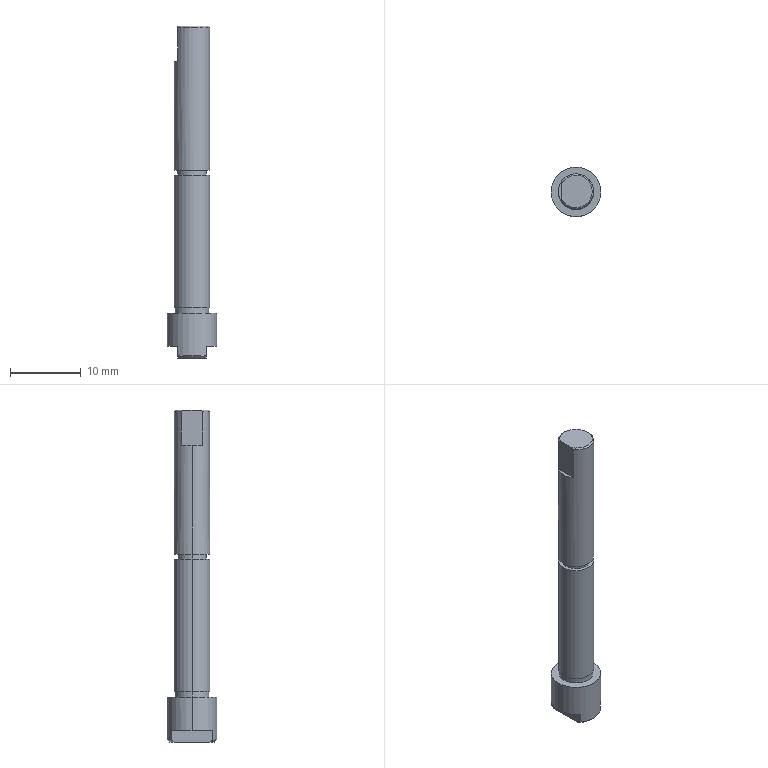Part | NX | 1 solid | 31 faces | box 7 x 7 x 46.9 mm | volume 962.4 mm3 | plane 12 | cylinder 12 | cone 7 | commonest cylinder face diameters 5 x4 2.5 x2 4 x2 4.8 x2 7 x2
STEP:
#1=CARTESIAN_POINT('',(-2.,1.136,41.07));
#2=VERTEX_POINT('',#1);
#3=CARTESIAN_POINT('',(-2.,-1.136,41.07));
#4=VERTEX_POINT('',#3);
#5=CARTESIAN_POINT('',(0.,0.,41.07));
#6=DIRECTION('',(0.,0.,-1.));
#7=DIRECTION('',(-1.,0.,0.));
#8=AXIS2_PLACEMENT_3D('',#5,#6,#7);
#9=CIRCLE('',#8,2.3);
#10=EDGE_CURVE('',#2,#4,#9,.T.);
#11=ORIENTED_EDGE('',*,*,#10,.F.);
#12=CARTESIAN_POINT('',(-2.,0.,41.07));
#13=DIRECTION('',(0.,1.,0.));
#14=VECTOR('',#13,1000.);
#15=LINE('',#12,#14);
#16=EDGE_CURVE('',#4,#2,#15,.T.);
#17=ORIENTED_EDGE('',*,*,#16,.F.);
#18=EDGE_LOOP('',(#11,#17));
#19=FACE_BOUND('',#18,.T.);
#20=CARTESIAN_POINT('',(0.,0.,41.07));
#21=DIRECTION('',(0.,0.,1.));
#22=DIRECTION('',(1.,0.,0.));
#23=AXIS2_PLACEMENT_3D('',#20,#21,#22);
#24=PLANE('',#23);
#25=ADVANCED_FACE('',(#19),#24,.T.);
#26=ORIENTED_EDGE('',*,*,#16,.T.);
#27=CARTESIAN_POINT('',(-2.,1.5,40.87));
#28=VERTEX_POINT('',#27);
#29=CARTESIAN_POINT('',(-2.,1.136,41.07));
#30=CARTESIAN_POINT('',(-2.,1.167,41.055));
#31=CARTESIAN_POINT('',(-2.,1.198,41.039));
#32=CARTESIAN_POINT('',(-2.,1.228,41.023));
#33=CARTESIAN_POINT('',(-2.,1.259,41.007));
#34=CARTESIAN_POINT('',(-2.,1.29,40.99));
#35=CARTESIAN_POINT('',(-2.,1.32,40.974));
#36=CARTESIAN_POINT('',(-2.,1.35,40.957));
#37=CARTESIAN_POINT('',(-2.,1.38,40.94));
#38=CARTESIAN_POINT('',(-2.,1.41,40.923));
#39=CARTESIAN_POINT('',(-2.,1.44,40.905));
#40=CARTESIAN_POINT('',(-2.,1.47,40.888));
#41=CARTESIAN_POINT('',(-2.,1.5,40.87));
#42=B_SPLINE_CURVE_WITH_KNOTS('',3,(#29,#30,#31,#32,#33,#34,#35,#36,#37,#38,#39,#40,#41),.UNSPECIFIED.,.F.,.F.,(4,3,3,3,4),(0.,0.1039,0.2078,0.3117,0.4156),.UNSPECIFIED.);
#43=EDGE_CURVE('',#2,#28,#42,.T.);
#44=ORIENTED_EDGE('',*,*,#43,.T.);
#45=CARTESIAN_POINT('',(-2.,1.5,36.07));
#46=VERTEX_POINT('',#45);
#47=CARTESIAN_POINT('',(-2.,1.5,0.));
#48=DIRECTION('',(0.,0.,1.));
#49=VECTOR('',#48,1000.);
#50=LINE('',#47,#49);
#51=EDGE_CURVE('',#46,#28,#50,.T.);
#52=ORIENTED_EDGE('',*,*,#51,.F.);
#53=CARTESIAN_POINT('',(-2.,-1.5,36.07));
#54=VERTEX_POINT('',#53);
#55=CARTESIAN_POINT('',(-2.,0.,36.07));
#56=DIRECTION('',(0.,-1.,0.));
#57=VECTOR('',#56,1000.);
#58=LINE('',#55,#57);
#59=EDGE_CURVE('',#46,#54,#58,.T.);
#60=ORIENTED_EDGE('',*,*,#59,.T.);
#61=CARTESIAN_POINT('',(-2.,-1.5,40.87));
#62=VERTEX_POINT('',#61);
#63=CARTESIAN_POINT('',(-2.,-1.5,0.));
#64=DIRECTION('',(0.,0.,1.));
#65=VECTOR('',#64,1000.);
#66=LINE('',#63,#65);
#67=EDGE_CURVE('',#54,#62,#66,.T.);
#68=ORIENTED_EDGE('',*,*,#67,.T.);
#69=CARTESIAN_POINT('',(-2.,-1.5,40.87));
#70=CARTESIAN_POINT('',(-2.,-1.47,40.888));
#71=CARTESIAN_POINT('',(-2.,-1.441,40.905));
#72=CARTESIAN_POINT('',(-2.,-1.411,40.923));
#73=CARTESIAN_POINT('',(-2.,-1.381,40.94));
#74=CARTESIAN_POINT('',(-2.,-1.35,40.957));
#75=CARTESIAN_POINT('',(-2.,-1.32,40.974));
#76=CARTESIAN_POINT('',(-2.,-1.29,40.99));
#77=CARTESIAN_POINT('',(-2.,-1.259,41.007));
#78=CARTESIAN_POINT('',(-2.,-1.228,41.023));
#79=CARTESIAN_POINT('',(-2.,-1.198,41.039));
#80=CARTESIAN_POINT('',(-2.,-1.167,41.055));
#81=CARTESIAN_POINT('',(-2.,-1.136,41.07));
#82=B_SPLINE_CURVE_WITH_KNOTS('',3,(#69,#70,#71,#72,#73,#74,#75,#76,#77,#78,#79,#80,#81),.UNSPECIFIED.,.F.,.F.,(4,3,3,3,4),(0.,0.1037,0.2076,0.3116,0.4156),.UNSPECIFIED.);
#83=EDGE_CURVE('',#62,#4,#82,.T.);
#84=ORIENTED_EDGE('',*,*,#83,.T.);
#85=EDGE_LOOP('',(#26,#44,#52,#60,#68,#84));
#86=FACE_BOUND('',#85,.T.);
#87=CARTESIAN_POINT('',(-2.,-3.316,38.));
#88=DIRECTION('',(1.,0.,0.));
#89=DIRECTION('',(0.,1.,0.));
#90=AXIS2_PLACEMENT_3D('',#87,#88,#89);
#91=PLANE('',#90);
#92=ADVANCED_FACE('',(#86),#91,.F.);
#93=CARTESIAN_POINT('',(-2.5,0.,36.07));
#94=VERTEX_POINT('',#93);
#95=CARTESIAN_POINT('',(0.,0.,36.07));
#96=DIRECTION('',(0.,0.,1.));
#97=DIRECTION('',(1.,0.,0.));
#98=AXIS2_PLACEMENT_3D('',#95,#96,#97);
#99=CIRCLE('',#98,2.5);
#100=EDGE_CURVE('',#94,#54,#99,.T.);
#101=ORIENTED_EDGE('',*,*,#100,.F.);
#102=CARTESIAN_POINT('',(-2.5,0.,20.7));
#103=VERTEX_POINT('',#102);
#104=CARTESIAN_POINT('',(-2.5,0.,0.));
#105=DIRECTION('',(0.,0.,1.));
#106=VECTOR('',#105,1000.);
#107=LINE('',#104,#106);
#108=EDGE_CURVE('',#103,#94,#107,.T.);
#109=ORIENTED_EDGE('',*,*,#108,.F.);
#110=CARTESIAN_POINT('',(2.5,0.,20.7));
#111=VERTEX_POINT('',#110);
#112=CARTESIAN_POINT('',(0.,0.,20.7));
#113=DIRECTION('',(0.,0.,1.));
#114=DIRECTION('',(1.,0.,0.));
#115=AXIS2_PLACEMENT_3D('',#112,#113,#114);
#116=CIRCLE('',#115,2.5);
#117=EDGE_CURVE('',#103,#111,#116,.T.);
#118=ORIENTED_EDGE('',*,*,#117,.T.);
#119=CARTESIAN_POINT('',(2.5,0.,40.87));
#120=VERTEX_POINT('',#119);
#121=CARTESIAN_POINT('',(2.5,0.,0.));
#122=DIRECTION('',(0.,0.,1.));
#123=VECTOR('',#122,1000.);
#124=LINE('',#121,#123);
#125=EDGE_CURVE('',#111,#120,#124,.T.);
#126=ORIENTED_EDGE('',*,*,#125,.T.);
#127=CARTESIAN_POINT('',(0.,0.,40.87));
#128=DIRECTION('',(0.,0.,-1.));
#129=DIRECTION('',(-1.,0.,0.));
#130=AXIS2_PLACEMENT_3D('',#127,#128,#129);
#131=CIRCLE('',#130,2.5);
#132=EDGE_CURVE('',#120,#62,#131,.T.);
#133=ORIENTED_EDGE('',*,*,#132,.T.);
#134=ORIENTED_EDGE('',*,*,#67,.F.);
#135=EDGE_LOOP('',(#101,#109,#118,#126,#133,#134));
#136=FACE_BOUND('',#135,.T.);
#137=CARTESIAN_POINT('',(0.,0.,0.));
#138=DIRECTION('',(0.,0.,1.));
#139=DIRECTION('',(1.,0.,0.));
#140=AXIS2_PLACEMENT_3D('',#137,#138,#139);
#141=CYLINDRICAL_SURFACE('',#140,2.5);
#142=ADVANCED_FACE('',(#136),#141,.T.);
#143=CARTESIAN_POINT('',(-2.,-2.498,-5.83));
#144=VERTEX_POINT('',#143);
#145=CARTESIAN_POINT('',(2.,-2.498,-5.83));
#146=VERTEX_POINT('',#145);
#147=CARTESIAN_POINT('',(0.,0.,-5.83));
#148=DIRECTION('',(0.,0.,1.));
#149=DIRECTION('',(1.,0.,0.));
#150=AXIS2_PLACEMENT_3D('',#147,#148,#149);
#151=CIRCLE('',#150,3.2);
#152=EDGE_CURVE('',#144,#146,#151,.T.);
#153=ORIENTED_EDGE('',*,*,#152,.T.);
#154=CARTESIAN_POINT('',(2.,-2.872,-5.53));
#155=VERTEX_POINT('',#154);
#156=CARTESIAN_POINT('',(2.,-2.872,-5.53));
#157=CARTESIAN_POINT('',(2.,-2.83,-5.565));
#158=CARTESIAN_POINT('',(2.,-2.745,-5.634));
#159=CARTESIAN_POINT('',(2.,-2.62,-5.734));
#160=CARTESIAN_POINT('',(2.,-2.539,-5.798));
#161=CARTESIAN_POINT('',(2.,-2.498,-5.83));
#162=B_SPLINE_CURVE_WITH_KNOTS('',3,(#156,#157,#158,#159,#160,#161),.UNSPECIFIED.,.F.,.F.,(4,1,1,4),(0.,0.3333,0.6667,1.),.UNSPECIFIED.);
#163=EDGE_CURVE('',#155,#146,#162,.T.);
#164=ORIENTED_EDGE('',*,*,#163,.F.);
#165=CARTESIAN_POINT('',(-2.,-2.872,-5.53));
#166=VERTEX_POINT('',#165);
#167=CARTESIAN_POINT('',(0.,0.,-5.53));
#168=DIRECTION('',(0.,0.,1.));
#169=DIRECTION('',(1.,0.,0.));
#170=AXIS2_PLACEMENT_3D('',#167,#168,#169);
#171=CIRCLE('',#170,3.5);
#172=EDGE_CURVE('',#166,#155,#171,.T.);
#173=ORIENTED_EDGE('',*,*,#172,.F.);
#174=CARTESIAN_POINT('',(-2.,-2.872,-5.53));
#175=CARTESIAN_POINT('',(-2.,-2.743,-5.636));
#176=CARTESIAN_POINT('',(-2.,-2.618,-5.736));
#177=CARTESIAN_POINT('',(-2.,-2.498,-5.83));
#178=B_SPLINE_CURVE_WITH_KNOTS('',3,(#174,#175,#176,#177),.UNSPECIFIED.,.F.,.F.,(4,4),(0.,1.),.UNSPECIFIED.);
#179=EDGE_CURVE('',#166,#144,#178,.T.);
#180=ORIENTED_EDGE('',*,*,#179,.T.);
#181=EDGE_LOOP('',(#153,#164,#173,#180));
#182=FACE_BOUND('',#181,.T.);
#183=CARTESIAN_POINT('',(0.,0.,-5.68));
#184=DIRECTION('',(0.,0.,1.));
#185=DIRECTION('',(1.,0.,0.));
#186=AXIS2_PLACEMENT_3D('',#183,#184,#185);
#187=CONICAL_SURFACE('',#186,3.35,0.7854);
#188=ADVANCED_FACE('',(#182),#187,.T.);
#189=ORIENTED_EDGE('',*,*,#100,.T.);
#190=ORIENTED_EDGE('',*,*,#59,.F.);
#191=CARTESIAN_POINT('',(0.,0.,36.07));
#192=DIRECTION('',(0.,0.,1.));
#193=DIRECTION('',(1.,0.,0.));
#194=AXIS2_PLACEMENT_3D('',#191,#192,#193);
#195=CIRCLE('',#194,2.5);
#196=EDGE_CURVE('',#46,#94,#195,.T.);
#197=ORIENTED_EDGE('',*,*,#196,.T.);
#198=EDGE_LOOP('',(#189,#190,#197));
#199=FACE_BOUND('',#198,.T.);
#200=CARTESIAN_POINT('',(0.,0.,36.07));
#201=DIRECTION('',(0.,0.,1.));
#202=DIRECTION('',(1.,0.,0.));
#203=AXIS2_PLACEMENT_3D('',#200,#201,#202);
#204=PLANE('',#203);
#205=ADVANCED_FACE('',(#199),#204,.T.);
#206=CARTESIAN_POINT('',(2.5,0.,20.));
#207=VERTEX_POINT('',#206);
#208=CARTESIAN_POINT('',(-2.5,0.,20.));
#209=VERTEX_POINT('',#208);
#210=CARTESIAN_POINT('',(0.,0.,20.));
#211=DIRECTION('',(0.,0.,1.));
#212=DIRECTION('',(1.,0.,0.));
#213=AXIS2_PLACEMENT_3D('',#210,#211,#212);
#214=CIRCLE('',#213,2.5);
#215=EDGE_CURVE('',#207,#209,#214,.T.);
#216=ORIENTED_EDGE('',*,*,#215,.T.);
#217=CARTESIAN_POINT('',(0.,0.,20.));
#218=DIRECTION('',(0.,0.,1.));
#219=DIRECTION('',(1.,0.,0.));
#220=AXIS2_PLACEMENT_3D('',#217,#218,#219);
#221=CIRCLE('',#220,2.5);
#222=EDGE_CURVE('',#209,#207,#221,.T.);
#223=ORIENTED_EDGE('',*,*,#222,.T.);
#224=EDGE_LOOP('',(#216,#223));
#225=FACE_BOUND('',#224,.T.);
#226=CARTESIAN_POINT('',(-2.,0.,20.));
#227=VERTEX_POINT('',#226);
#228=CARTESIAN_POINT('',(2.,0.,20.));
#229=VERTEX_POINT('',#228);
#230=CARTESIAN_POINT('',(0.,0.,20.));
#231=DIRECTION('',(0.,0.,-1.));
#232=DIRECTION('',(-1.,0.,0.));
#233=AXIS2_PLACEMENT_3D('',#230,#231,#232);
#234=CIRCLE('',#233,2.);
#235=EDGE_CURVE('',#227,#229,#234,.T.);
#236=ORIENTED_EDGE('',*,*,#235,.T.);
#237=CARTESIAN_POINT('',(0.,0.,20.));
#238=DIRECTION('',(0.,0.,-1.));
#239=DIRECTION('',(-1.,0.,0.));
#240=AXIS2_PLACEMENT_3D('',#237,#238,#239);
#241=CIRCLE('',#240,2.);
#242=EDGE_CURVE('',#229,#227,#241,.T.);
#243=ORIENTED_EDGE('',*,*,#242,.T.);
#244=EDGE_LOOP('',(#236,#243));
#245=FACE_BOUND('',#244,.T.);
#246=CARTESIAN_POINT('',(0.,0.,20.));
#247=DIRECTION('',(0.,0.,-1.));
#248=DIRECTION('',(0.,-1.,0.));
#249=AXIS2_PLACEMENT_3D('',#246,#247,#248);
#250=PLANE('',#249);
#251=ADVANCED_FACE('',(#225,#245),#250,.F.);
#252=ORIENTED_EDGE('',*,*,#235,.F.);
#253=CARTESIAN_POINT('',(-2.,0.,20.7));
#254=VERTEX_POINT('',#253);
#255=CARTESIAN_POINT('',(-2.,0.,20.683));
#256=DIRECTION('',(0.,0.,-1.));
#257=VECTOR('',#256,1000.);
#258=LINE('',#255,#257);
#259=EDGE_CURVE('',#227,#254,#258,.F.);
#260=ORIENTED_EDGE('',*,*,#259,.T.);
#261=CARTESIAN_POINT('',(2.,0.,20.7));
#262=VERTEX_POINT('',#261);
#263=CARTESIAN_POINT('',(0.,0.,20.7));
#264=DIRECTION('',(0.,0.,-1.));
#265=DIRECTION('',(-1.,0.,0.));
#266=AXIS2_PLACEMENT_3D('',#263,#264,#265);
#267=CIRCLE('',#266,2.);
#268=EDGE_CURVE('',#254,#262,#267,.T.);
#269=ORIENTED_EDGE('',*,*,#268,.T.);
#270=CARTESIAN_POINT('',(2.,0.,20.683));
#271=DIRECTION('',(0.,0.,-1.));
#272=VECTOR('',#271,1000.);
#273=LINE('',#270,#272);
#274=EDGE_CURVE('',#229,#262,#273,.F.);
#275=ORIENTED_EDGE('',*,*,#274,.F.);
#276=EDGE_LOOP('',(#252,#260,#269,#275));
#277=FACE_BOUND('',#276,.T.);
#278=CARTESIAN_POINT('',(0.,0.,20.683));
#279=DIRECTION('',(0.,0.,-1.));
#280=DIRECTION('',(-1.,0.,0.));
#281=AXIS2_PLACEMENT_3D('',#278,#279,#280);
#282=CYLINDRICAL_SURFACE('',#281,2.);
#283=ADVANCED_FACE('',(#277),#282,.T.);
#284=CARTESIAN_POINT('',(2.,2.498,-5.83));
#285=VERTEX_POINT('',#284);
#286=CARTESIAN_POINT('',(2.,0.,-5.83));
#287=DIRECTION('',(0.,-1.,0.));
#288=VECTOR('',#287,1000.);
#289=LINE('',#286,#288);
#290=EDGE_CURVE('',#285,#146,#289,.T.);
#291=ORIENTED_EDGE('',*,*,#290,.T.);
#292=ORIENTED_EDGE('',*,*,#152,.F.);
#293=CARTESIAN_POINT('',(-2.,2.498,-5.83));
#294=VERTEX_POINT('',#293);
#295=CARTESIAN_POINT('',(-2.,0.,-5.83));
#296=DIRECTION('',(0.,1.,0.));
#297=VECTOR('',#296,1000.);
#298=LINE('',#295,#297);
#299=EDGE_CURVE('',#144,#294,#298,.T.);
#300=ORIENTED_EDGE('',*,*,#299,.T.);
#301=CARTESIAN_POINT('',(0.,0.,-5.83));
#302=DIRECTION('',(0.,0.,1.));
#303=DIRECTION('',(1.,0.,0.));
#304=AXIS2_PLACEMENT_3D('',#301,#302,#303);
#305=CIRCLE('',#304,3.2);
#306=EDGE_CURVE('',#285,#294,#305,.T.);
#307=ORIENTED_EDGE('',*,*,#306,.F.);
#308=EDGE_LOOP('',(#291,#292,#300,#307));
#309=FACE_BOUND('',#308,.T.);
#310=CARTESIAN_POINT('',(1.7,0.,-5.83));
#311=VERTEX_POINT('',#310);
#312=CARTESIAN_POINT('',(-1.7,0.,-5.83));
#313=VERTEX_POINT('',#312);
#314=CARTESIAN_POINT('',(0.,0.,-5.83));
#315=DIRECTION('',(0.,0.,-1.));
#316=DIRECTION('',(-1.,0.,0.));
#317=AXIS2_PLACEMENT_3D('',#314,#315,#316);
#318=CIRCLE('',#317,1.7);
#319=EDGE_CURVE('',#311,#313,#318,.T.);
#320=ORIENTED_EDGE('',*,*,#319,.F.);
#321=CARTESIAN_POINT('',(0.,0.,-5.83));
#322=DIRECTION('',(0.,0.,-1.));
#323=DIRECTION('',(-1.,0.,0.));
#324=AXIS2_PLACEMENT_3D('',#321,#322,#323);
#325=CIRCLE('',#324,1.7);
#326=EDGE_CURVE('',#313,#311,#325,.T.);
#327=ORIENTED_EDGE('',*,*,#326,.F.);
#328=EDGE_LOOP('',(#320,#327));
#329=FACE_BOUND('',#328,.T.);
#330=CARTESIAN_POINT('',(0.,0.,-5.83));
#331=DIRECTION('',(0.,0.,-1.));
#332=DIRECTION('',(0.,-1.,0.));
#333=AXIS2_PLACEMENT_3D('',#330,#331,#332);
#334=PLANE('',#333);
#335=ADVANCED_FACE('',(#309,#329),#334,.T.);
#336=ORIENTED_EDGE('',*,*,#117,.F.);
#337=CARTESIAN_POINT('',(0.,0.,20.7));
#338=DIRECTION('',(0.,0.,1.));
#339=DIRECTION('',(1.,0.,0.));
#340=AXIS2_PLACEMENT_3D('',#337,#338,#339);
#341=CIRCLE('',#340,2.5);
#342=EDGE_CURVE('',#111,#103,#341,.T.);
#343=ORIENTED_EDGE('',*,*,#342,.F.);
#344=EDGE_LOOP('',(#336,#343));
#345=FACE_BOUND('',#344,.T.);
#346=CARTESIAN_POINT('',(0.,0.,20.7));
#347=DIRECTION('',(0.,0.,-1.));
#348=DIRECTION('',(-1.,0.,0.));
#349=AXIS2_PLACEMENT_3D('',#346,#347,#348);
#350=CIRCLE('',#349,2.);
#351=EDGE_CURVE('',#262,#254,#350,.T.);
#352=ORIENTED_EDGE('',*,*,#351,.F.);
#353=ORIENTED_EDGE('',*,*,#268,.F.);
#354=EDGE_LOOP('',(#352,#353));
#355=FACE_BOUND('',#354,.T.);
#356=CARTESIAN_POINT('',(0.,0.,20.7));
#357=DIRECTION('',(0.,0.,-1.));
#358=DIRECTION('',(0.,-1.,0.));
#359=AXIS2_PLACEMENT_3D('',#356,#357,#358);
#360=PLANE('',#359);
#361=ADVANCED_FACE('',(#345,#355),#360,.T.);
#362=ORIENTED_EDGE('',*,*,#215,.F.);
#363=CARTESIAN_POINT('',(2.5,0.,1.3));
#364=VERTEX_POINT('',#363);
#365=CARTESIAN_POINT('',(2.5,0.,0.));
#366=DIRECTION('',(0.,0.,1.));
#367=VECTOR('',#366,1000.);
#368=LINE('',#365,#367);
#369=EDGE_CURVE('',#364,#207,#368,.T.);
#370=ORIENTED_EDGE('',*,*,#369,.F.);
#371=CARTESIAN_POINT('',(-2.5,0.,1.3));
#372=VERTEX_POINT('',#371);
#373=CARTESIAN_POINT('',(0.,0.,1.3));
#374=DIRECTION('',(0.,0.,1.));
#375=DIRECTION('',(1.,0.,0.));
#376=AXIS2_PLACEMENT_3D('',#373,#374,#375);
#377=CIRCLE('',#376,2.5);
#378=EDGE_CURVE('',#364,#372,#377,.T.);
#379=ORIENTED_EDGE('',*,*,#378,.T.);
#380=CARTESIAN_POINT('',(-2.5,0.,0.));
#381=DIRECTION('',(0.,0.,1.));
#382=VECTOR('',#381,1000.);
#383=LINE('',#380,#382);
#384=EDGE_CURVE('',#372,#209,#383,.T.);
#385=ORIENTED_EDGE('',*,*,#384,.T.);
#386=EDGE_LOOP('',(#362,#370,#379,#385));
#387=FACE_BOUND('',#386,.T.);
#388=CARTESIAN_POINT('',(0.,0.,0.));
#389=DIRECTION('',(0.,0.,1.));
#390=DIRECTION('',(1.,0.,0.));
#391=AXIS2_PLACEMENT_3D('',#388,#389,#390);
#392=CYLINDRICAL_SURFACE('',#391,2.5);
#393=ADVANCED_FACE('',(#387),#392,.T.);
#394=CARTESIAN_POINT('',(3.5,0.,0.5));
#395=VERTEX_POINT('',#394);
#396=CARTESIAN_POINT('',(-3.5,0.,0.5));
#397=VERTEX_POINT('',#396);
#398=CARTESIAN_POINT('',(0.,0.,0.5));
#399=DIRECTION('',(0.,0.,-1.));
#400=DIRECTION('',(-1.,0.,0.));
#401=AXIS2_PLACEMENT_3D('',#398,#399,#400);
#402=CIRCLE('',#401,3.5);
#403=EDGE_CURVE('',#395,#397,#402,.T.);
#404=ORIENTED_EDGE('',*,*,#403,.F.);
#405=CARTESIAN_POINT('',(0.,0.,0.5));
#406=DIRECTION('',(0.,0.,-1.));
#407=DIRECTION('',(-1.,0.,0.));
#408=AXIS2_PLACEMENT_3D('',#405,#406,#407);
#409=CIRCLE('',#408,3.5);
#410=EDGE_CURVE('',#397,#395,#409,.T.);
#411=ORIENTED_EDGE('',*,*,#410,.F.);
#412=EDGE_LOOP('',(#404,#411));
#413=FACE_BOUND('',#412,.T.);
#414=CARTESIAN_POINT('',(-2.4,0.,0.5));
#415=VERTEX_POINT('',#414);
#416=CARTESIAN_POINT('',(2.4,0.,0.5));
#417=VERTEX_POINT('',#416);
#418=CARTESIAN_POINT('',(0.,0.,0.5));
#419=DIRECTION('',(0.,0.,-1.));
#420=DIRECTION('',(1.,0.,0.));
#421=AXIS2_PLACEMENT_3D('',#418,#419,#420);
#422=CIRCLE('',#421,2.4);
#423=EDGE_CURVE('',#415,#417,#422,.T.);
#424=ORIENTED_EDGE('',*,*,#423,.T.);
#425=CARTESIAN_POINT('',(0.,0.,0.5));
#426=DIRECTION('',(0.,0.,-1.));
#427=DIRECTION('',(1.,0.,0.));
#428=AXIS2_PLACEMENT_3D('',#425,#426,#427);
#429=CIRCLE('',#428,2.4);
#430=EDGE_CURVE('',#417,#415,#429,.T.);
#431=ORIENTED_EDGE('',*,*,#430,.T.);
#432=EDGE_LOOP('',(#424,#431));
#433=FACE_BOUND('',#432,.T.);
#434=CARTESIAN_POINT('',(0.,0.,0.5));
#435=DIRECTION('',(0.,0.,-1.));
#436=DIRECTION('',(0.,-1.,0.));
#437=AXIS2_PLACEMENT_3D('',#434,#435,#436);
#438=PLANE('',#437);
#439=ADVANCED_FACE('',(#413,#433),#438,.F.);
#440=ORIENTED_EDGE('',*,*,#290,.F.);
#441=CARTESIAN_POINT('',(2.,2.872,-5.53));
#442=VERTEX_POINT('',#441);
#443=CARTESIAN_POINT('',(2.,2.872,-5.53));
#444=CARTESIAN_POINT('',(2.,2.743,-5.636));
#445=CARTESIAN_POINT('',(2.,2.618,-5.736));
#446=CARTESIAN_POINT('',(2.,2.498,-5.83));
#447=B_SPLINE_CURVE_WITH_KNOTS('',3,(#443,#444,#445,#446),.UNSPECIFIED.,.F.,.F.,(4,4),(0.,1.),.UNSPECIFIED.);
#448=EDGE_CURVE('',#442,#285,#447,.T.);
#449=ORIENTED_EDGE('',*,*,#448,.F.);
#450=CARTESIAN_POINT('',(2.,2.872,-4.18));
#451=VERTEX_POINT('',#450);
#452=CARTESIAN_POINT('',(2.,2.872,0.));
#453=DIRECTION('',(0.,0.,-1.));
#454=VECTOR('',#453,1000.);
#455=LINE('',#452,#454);
#456=EDGE_CURVE('',#451,#442,#455,.T.);
#457=ORIENTED_EDGE('',*,*,#456,.F.);
#458=CARTESIAN_POINT('',(2.,-2.872,-4.18));
#459=VERTEX_POINT('',#458);
#460=CARTESIAN_POINT('',(2.,2.872,-4.18));
#461=DIRECTION('',(0.,-1.,0.));
#462=VECTOR('',#461,1000.);
#463=LINE('',#460,#462);
#464=EDGE_CURVE('',#451,#459,#463,.T.);
#465=ORIENTED_EDGE('',*,*,#464,.T.);
#466=CARTESIAN_POINT('',(2.,-2.872,0.));
#467=DIRECTION('',(0.,0.,-1.));
#468=VECTOR('',#467,1000.);
#469=LINE('',#466,#468);
#470=EDGE_CURVE('',#459,#155,#469,.T.);
#471=ORIENTED_EDGE('',*,*,#470,.T.);
#472=ORIENTED_EDGE('',*,*,#163,.T.);
#473=EDGE_LOOP('',(#440,#449,#457,#465,#471,#472));
#474=FACE_BOUND('',#473,.T.);
#475=CARTESIAN_POINT('',(2.,-2.872,-5.83));
#476=DIRECTION('',(-1.,0.,0.));
#477=DIRECTION('',(0.,0.,1.));
#478=AXIS2_PLACEMENT_3D('',#475,#476,#477);
#479=PLANE('',#478);
#480=ADVANCED_FACE('',(#474),#479,.F.);
#481=CARTESIAN_POINT('',(-2.4,0.,1.3));
#482=VERTEX_POINT('',#481);
#483=CARTESIAN_POINT('',(2.4,0.,1.3));
#484=VERTEX_POINT('',#483);
#485=CARTESIAN_POINT('',(0.,0.,1.3));
#486=DIRECTION('',(0.,0.,-1.));
#487=DIRECTION('',(1.,0.,0.));
#488=AXIS2_PLACEMENT_3D('',#485,#486,#487);
#489=CIRCLE('',#488,2.4);
#490=EDGE_CURVE('',#482,#484,#489,.T.);
#491=ORIENTED_EDGE('',*,*,#490,.T.);
#492=CARTESIAN_POINT('',(2.4,0.,0.315));
#493=DIRECTION('',(0.,0.,-1.));
#494=VECTOR('',#493,1000.);
#495=LINE('',#492,#494);
#496=EDGE_CURVE('',#484,#417,#495,.T.);
#497=ORIENTED_EDGE('',*,*,#496,.T.);
#498=ORIENTED_EDGE('',*,*,#423,.F.);
#499=CARTESIAN_POINT('',(-2.4,0.,0.315));
#500=DIRECTION('',(0.,0.,-1.));
#501=VECTOR('',#500,1000.);
#502=LINE('',#499,#501);
#503=EDGE_CURVE('',#482,#415,#502,.T.);
#504=ORIENTED_EDGE('',*,*,#503,.F.);
#505=EDGE_LOOP('',(#491,#497,#498,#504));
#506=FACE_BOUND('',#505,.T.);
#507=CARTESIAN_POINT('',(0.,0.,0.315));
#508=DIRECTION('',(0.,0.,-1.));
#509=DIRECTION('',(1.,0.,0.));
#510=AXIS2_PLACEMENT_3D('',#507,#508,#509);
#511=CYLINDRICAL_SURFACE('',#510,2.4);
#512=ADVANCED_FACE('',(#506),#511,.T.);
#513=ORIENTED_EDGE('',*,*,#299,.F.);
#514=ORIENTED_EDGE('',*,*,#179,.F.);
#515=CARTESIAN_POINT('',(-2.,-2.872,-4.18));
#516=VERTEX_POINT('',#515);
#517=CARTESIAN_POINT('',(-2.,-2.872,0.));
#518=DIRECTION('',(0.,0.,-1.));
#519=VECTOR('',#518,1000.);
#520=LINE('',#517,#519);
#521=EDGE_CURVE('',#516,#166,#520,.T.);
#522=ORIENTED_EDGE('',*,*,#521,.F.);
#523=CARTESIAN_POINT('',(-2.,2.872,-4.18));
#524=VERTEX_POINT('',#523);
#525=CARTESIAN_POINT('',(-2.,-2.872,-4.18));
#526=DIRECTION('',(0.,1.,0.));
#527=VECTOR('',#526,1000.);
#528=LINE('',#525,#527);
#529=EDGE_CURVE('',#516,#524,#528,.T.);
#530=ORIENTED_EDGE('',*,*,#529,.T.);
#531=CARTESIAN_POINT('',(-2.,2.872,-5.53));
#532=VERTEX_POINT('',#531);
#533=CARTESIAN_POINT('',(-2.,2.872,0.));
#534=DIRECTION('',(0.,0.,-1.));
#535=VECTOR('',#534,1000.);
#536=LINE('',#533,#535);
#537=EDGE_CURVE('',#524,#532,#536,.T.);
#538=ORIENTED_EDGE('',*,*,#537,.T.);
#539=CARTESIAN_POINT('',(-2.,2.872,-5.53));
#540=CARTESIAN_POINT('',(-2.,2.83,-5.565));
#541=CARTESIAN_POINT('',(-2.,2.745,-5.634));
#542=CARTESIAN_POINT('',(-2.,2.62,-5.734));
#543=CARTESIAN_POINT('',(-2.,2.539,-5.798));
#544=CARTESIAN_POINT('',(-2.,2.498,-5.83));
#545=B_SPLINE_CURVE_WITH_KNOTS('',3,(#539,#540,#541,#542,#543,#544),.UNSPECIFIED.,.F.,.F.,(4,1,1,4),(0.,0.3333,0.6667,1.),.UNSPECIFIED.);
#546=EDGE_CURVE('',#532,#294,#545,.T.);
#547=ORIENTED_EDGE('',*,*,#546,.T.);
#548=EDGE_LOOP('',(#513,#514,#522,#530,#538,#547));
#549=FACE_BOUND('',#548,.T.);
#550=CARTESIAN_POINT('',(-2.,2.872,-5.83));
#551=DIRECTION('',(1.,0.,0.));
#552=DIRECTION('',(0.,1.,0.));
#553=AXIS2_PLACEMENT_3D('',#550,#551,#552);
#554=PLANE('',#553);
#555=ADVANCED_FACE('',(#549),#554,.F.);
#556=ORIENTED_EDGE('',*,*,#378,.F.);
#557=CARTESIAN_POINT('',(0.,0.,1.3));
#558=DIRECTION('',(0.,0.,1.));
#559=DIRECTION('',(1.,0.,0.));
#560=AXIS2_PLACEMENT_3D('',#557,#558,#559);
#561=CIRCLE('',#560,2.5);
#562=EDGE_CURVE('',#372,#364,#561,.T.);
#563=ORIENTED_EDGE('',*,*,#562,.F.);
#564=EDGE_LOOP('',(#556,#563));
#565=FACE_BOUND('',#564,.T.);
#566=ORIENTED_EDGE('',*,*,#490,.F.);
#567=CARTESIAN_POINT('',(0.,0.,1.3));
#568=DIRECTION('',(0.,0.,-1.));
#569=DIRECTION('',(1.,0.,0.));
#570=AXIS2_PLACEMENT_3D('',#567,#568,#569);
#571=CIRCLE('',#570,2.4);
#572=EDGE_CURVE('',#484,#482,#571,.T.);
#573=ORIENTED_EDGE('',*,*,#572,.F.);
#574=EDGE_LOOP('',(#566,#573));
#575=FACE_BOUND('',#574,.T.);
#576=CARTESIAN_POINT('',(0.,0.,1.3));
#577=DIRECTION('',(0.,0.,-1.));
#578=DIRECTION('',(0.,-1.,0.));
#579=AXIS2_PLACEMENT_3D('',#576,#577,#578);
#580=PLANE('',#579);
#581=ADVANCED_FACE('',(#565,#575),#580,.T.);
#582=CARTESIAN_POINT('',(-3.5,0.,-4.18));
#583=VERTEX_POINT('',#582);
#584=CARTESIAN_POINT('',(0.,0.,-4.18));
#585=DIRECTION('',(0.,0.,-1.));
#586=DIRECTION('',(-1.,0.,0.));
#587=AXIS2_PLACEMENT_3D('',#584,#585,#586);
#588=CIRCLE('',#587,3.5);
#589=EDGE_CURVE('',#583,#524,#588,.T.);
#590=ORIENTED_EDGE('',*,*,#589,.F.);
#591=CARTESIAN_POINT('',(-3.5,0.,0.));
#592=DIRECTION('',(0.,0.,-1.));
#593=VECTOR('',#592,1000.);
#594=LINE('',#591,#593);
#595=EDGE_CURVE('',#583,#397,#594,.F.);
#596=ORIENTED_EDGE('',*,*,#595,.T.);
#597=ORIENTED_EDGE('',*,*,#410,.T.);
#598=CARTESIAN_POINT('',(3.5,0.,-4.18));
#599=VERTEX_POINT('',#598);
#600=CARTESIAN_POINT('',(3.5,0.,0.));
#601=DIRECTION('',(0.,0.,-1.));
#602=VECTOR('',#601,1000.);
#603=LINE('',#600,#602);
#604=EDGE_CURVE('',#599,#395,#603,.F.);
#605=ORIENTED_EDGE('',*,*,#604,.F.);
#606=CARTESIAN_POINT('',(0.,0.,-4.18));
#607=DIRECTION('',(0.,0.,-1.));
#608=DIRECTION('',(-1.,0.,0.));
#609=AXIS2_PLACEMENT_3D('',#606,#607,#608);
#610=CIRCLE('',#609,3.5);
#611=EDGE_CURVE('',#451,#599,#610,.T.);
#612=ORIENTED_EDGE('',*,*,#611,.F.);
#613=ORIENTED_EDGE('',*,*,#456,.T.);
#614=CARTESIAN_POINT('',(0.,0.,-5.53));
#615=DIRECTION('',(0.,0.,1.));
#616=DIRECTION('',(1.,0.,0.));
#617=AXIS2_PLACEMENT_3D('',#614,#615,#616);
#618=CIRCLE('',#617,3.5);
#619=EDGE_CURVE('',#442,#532,#618,.T.);
#620=ORIENTED_EDGE('',*,*,#619,.T.);
#621=ORIENTED_EDGE('',*,*,#537,.F.);
#622=EDGE_LOOP('',(#590,#596,#597,#605,#612,#613,#620,#621));
#623=FACE_BOUND('',#622,.T.);
#624=CARTESIAN_POINT('',(0.,0.,0.));
#625=DIRECTION('',(0.,0.,-1.));
#626=DIRECTION('',(-1.,0.,0.));
#627=AXIS2_PLACEMENT_3D('',#624,#625,#626);
#628=CYLINDRICAL_SURFACE('',#627,3.5);
#629=ADVANCED_FACE('',(#623),#628,.T.);
#630=ORIENTED_EDGE('',*,*,#589,.T.);
#631=ORIENTED_EDGE('',*,*,#529,.F.);
#632=CARTESIAN_POINT('',(0.,0.,-4.18));
#633=DIRECTION('',(0.,0.,-1.));
#634=DIRECTION('',(-1.,0.,0.));
#635=AXIS2_PLACEMENT_3D('',#632,#633,#634);
#636=CIRCLE('',#635,3.5);
#637=EDGE_CURVE('',#516,#583,#636,.T.);
#638=ORIENTED_EDGE('',*,*,#637,.T.);
#639=EDGE_LOOP('',(#630,#631,#638));
#640=FACE_BOUND('',#639,.T.);
#641=CARTESIAN_POINT('',(0.,0.,-4.18));
#642=DIRECTION('',(0.,0.,-1.));
#643=DIRECTION('',(0.,-1.,0.));
#644=AXIS2_PLACEMENT_3D('',#641,#642,#643);
#645=PLANE('',#644);
#646=ADVANCED_FACE('',(#640),#645,.T.);
#647=ORIENTED_EDGE('',*,*,#306,.T.);
#648=ORIENTED_EDGE('',*,*,#546,.F.);
#649=ORIENTED_EDGE('',*,*,#619,.F.);
#650=ORIENTED_EDGE('',*,*,#448,.T.);
#651=EDGE_LOOP('',(#647,#648,#649,#650));
#652=FACE_BOUND('',#651,.T.);
#653=CARTESIAN_POINT('',(0.,0.,-5.68));
#654=DIRECTION('',(0.,0.,1.));
#655=DIRECTION('',(1.,0.,0.));
#656=AXIS2_PLACEMENT_3D('',#653,#654,#655);
#657=CONICAL_SURFACE('',#656,3.35,0.7854);
#658=ADVANCED_FACE('',(#652),#657,.T.);
#659=CARTESIAN_POINT('',(0.,0.,-4.18));
#660=DIRECTION('',(0.,0.,-1.));
#661=DIRECTION('',(-1.,0.,0.));
#662=AXIS2_PLACEMENT_3D('',#659,#660,#661);
#663=CIRCLE('',#662,3.5);
#664=EDGE_CURVE('',#599,#459,#663,.T.);
#665=ORIENTED_EDGE('',*,*,#664,.T.);
#666=ORIENTED_EDGE('',*,*,#464,.F.);
#667=ORIENTED_EDGE('',*,*,#611,.T.);
#668=EDGE_LOOP('',(#665,#666,#667));
#669=FACE_BOUND('',#668,.T.);
#670=CARTESIAN_POINT('',(0.,0.,-4.18));
#671=DIRECTION('',(0.,0.,-1.));
#672=DIRECTION('',(0.,-1.,0.));
#673=AXIS2_PLACEMENT_3D('',#670,#671,#672);
#674=PLANE('',#673);
#675=ADVANCED_FACE('',(#669),#674,.T.);
#676=CARTESIAN_POINT('',(1.25,0.,3.17));
#677=VERTEX_POINT('',#676);
#678=CARTESIAN_POINT('',(-1.25,0.,3.17));
#679=VERTEX_POINT('',#678);
#680=CARTESIAN_POINT('',(0.,0.,3.17));
#681=DIRECTION('',(0.,0.,-1.));
#682=DIRECTION('',(-1.,0.,0.));
#683=AXIS2_PLACEMENT_3D('',#680,#681,#682);
#684=CIRCLE('',#683,1.25);
#685=EDGE_CURVE('',#677,#679,#684,.T.);
#686=ORIENTED_EDGE('',*,*,#685,.F.);
#687=CARTESIAN_POINT('',(1.25,0.,-5.57));
#688=VERTEX_POINT('',#687);
#689=CARTESIAN_POINT('',(1.25,0.,-5.83));
#690=DIRECTION('',(0.,0.,-1.));
#691=VECTOR('',#690,1000.);
#692=LINE('',#689,#691);
#693=EDGE_CURVE('',#677,#688,#692,.T.);
#694=ORIENTED_EDGE('',*,*,#693,.T.);
#695=CARTESIAN_POINT('',(-1.25,0.,-5.57));
#696=VERTEX_POINT('',#695);
#697=CARTESIAN_POINT('',(0.,0.,-5.57));
#698=DIRECTION('',(0.,0.,-1.));
#699=DIRECTION('',(-1.,0.,0.));
#700=AXIS2_PLACEMENT_3D('',#697,#698,#699);
#701=CIRCLE('',#700,1.25);
#702=EDGE_CURVE('',#688,#696,#701,.T.);
#703=ORIENTED_EDGE('',*,*,#702,.T.);
#704=CARTESIAN_POINT('',(-1.25,0.,-5.83));
#705=DIRECTION('',(0.,0.,-1.));
#706=VECTOR('',#705,1000.);
#707=LINE('',#704,#706);
#708=EDGE_CURVE('',#679,#696,#707,.T.);
#709=ORIENTED_EDGE('',*,*,#708,.F.);
#710=EDGE_LOOP('',(#686,#694,#703,#709));
#711=FACE_BOUND('',#710,.T.);
#712=CARTESIAN_POINT('',(0.,0.,-5.83));
#713=DIRECTION('',(0.,0.,-1.));
#714=DIRECTION('',(-1.,0.,0.));
#715=AXIS2_PLACEMENT_3D('',#712,#713,#714);
#716=CYLINDRICAL_SURFACE('',#715,1.25);
#717=ADVANCED_FACE('',(#711),#716,.F.);
#718=ORIENTED_EDGE('',*,*,#10,.T.);
#719=ORIENTED_EDGE('',*,*,#83,.F.);
#720=ORIENTED_EDGE('',*,*,#132,.F.);
#721=CARTESIAN_POINT('',(0.,0.,40.87));
#722=DIRECTION('',(0.,0.,-1.));
#723=DIRECTION('',(-1.,0.,0.));
#724=AXIS2_PLACEMENT_3D('',#721,#722,#723);
#725=CIRCLE('',#724,2.5);
#726=EDGE_CURVE('',#28,#120,#725,.T.);
#727=ORIENTED_EDGE('',*,*,#726,.F.);
#728=ORIENTED_EDGE('',*,*,#43,.F.);
#729=EDGE_LOOP('',(#718,#719,#720,#727,#728));
#730=FACE_BOUND('',#729,.T.);
#731=CARTESIAN_POINT('',(0.,0.,41.07));
#732=DIRECTION('',(0.,0.,-1.));
#733=DIRECTION('',(-1.,0.,0.));
#734=AXIS2_PLACEMENT_3D('',#731,#732,#733);
#735=CONICAL_SURFACE('',#734,2.3,0.7854);
#736=ADVANCED_FACE('',(#730),#735,.T.);
#737=ORIENTED_EDGE('',*,*,#685,.T.);
#738=CARTESIAN_POINT('',(0.,0.,3.921));
#739=VERTEX_POINT('',#738);
#740=CARTESIAN_POINT('',(-1.25,0.,3.17));
#741=DIRECTION('',(-0.8572,0.,-0.515));
#742=VECTOR('',#741,1000.);
#743=LINE('',#740,#742);
#744=EDGE_CURVE('',#739,#679,#743,.T.);
#745=ORIENTED_EDGE('',*,*,#744,.F.);
#746=CARTESIAN_POINT('',(1.25,0.,3.17));
#747=DIRECTION('',(0.8572,0.,-0.515));
#748=VECTOR('',#747,1000.);
#749=LINE('',#746,#748);
#750=EDGE_CURVE('',#739,#677,#749,.T.);
#751=ORIENTED_EDGE('',*,*,#750,.T.);
#752=EDGE_LOOP('',(#737,#745,#751));
#753=FACE_BOUND('',#752,.T.);
#754=CARTESIAN_POINT('',(0.,0.,3.17));
#755=DIRECTION('',(0.,0.,-1.));
#756=DIRECTION('',(-1.,0.,0.));
#757=AXIS2_PLACEMENT_3D('',#754,#755,#756);
#758=CONICAL_SURFACE('',#757,1.25,1.03);
#759=ADVANCED_FACE('',(#753),#758,.F.);
#760=ORIENTED_EDGE('',*,*,#319,.T.);
#761=CARTESIAN_POINT('',(-1.25,0.,-5.57));
#762=DIRECTION('',(-0.866,0.,-0.5));
#763=VECTOR('',#762,1000.);
#764=LINE('',#761,#763);
#765=EDGE_CURVE('',#313,#696,#764,.F.);
#766=ORIENTED_EDGE('',*,*,#765,.T.);
#767=ORIENTED_EDGE('',*,*,#702,.F.);
#768=CARTESIAN_POINT('',(1.25,0.,-5.57));
#769=DIRECTION('',(0.866,0.,-0.5));
#770=VECTOR('',#769,1000.);
#771=LINE('',#768,#770);
#772=EDGE_CURVE('',#311,#688,#771,.F.);
#773=ORIENTED_EDGE('',*,*,#772,.F.);
#774=EDGE_LOOP('',(#760,#766,#767,#773));
#775=FACE_BOUND('',#774,.T.);
#776=CARTESIAN_POINT('',(0.,0.,-5.57));
#777=DIRECTION('',(0.,0.,-1.));
#778=DIRECTION('',(-1.,0.,0.));
#779=AXIS2_PLACEMENT_3D('',#776,#777,#778);
#780=CONICAL_SURFACE('',#779,1.25,1.047);
#781=ADVANCED_FACE('',(#775),#780,.F.);
#782=CARTESIAN_POINT('',(0.,0.,-5.57));
#783=DIRECTION('',(0.,0.,-1.));
#784=DIRECTION('',(-1.,0.,0.));
#785=AXIS2_PLACEMENT_3D('',#782,#783,#784);
#786=CIRCLE('',#785,1.25);
#787=EDGE_CURVE('',#696,#688,#786,.T.);
#788=ORIENTED_EDGE('',*,*,#787,.F.);
#789=ORIENTED_EDGE('',*,*,#765,.F.);
#790=ORIENTED_EDGE('',*,*,#326,.T.);
#791=ORIENTED_EDGE('',*,*,#772,.T.);
#792=EDGE_LOOP('',(#788,#789,#790,#791));
#793=FACE_BOUND('',#792,.T.);
#794=CARTESIAN_POINT('',(0.,0.,-5.57));
#795=DIRECTION('',(0.,0.,-1.));
#796=DIRECTION('',(-1.,0.,0.));
#797=AXIS2_PLACEMENT_3D('',#794,#795,#796);
#798=CONICAL_SURFACE('',#797,1.25,1.047);
#799=ADVANCED_FACE('',(#793),#798,.F.);
#800=ORIENTED_EDGE('',*,*,#496,.F.);
#801=ORIENTED_EDGE('',*,*,#572,.T.);
#802=ORIENTED_EDGE('',*,*,#503,.T.);
#803=ORIENTED_EDGE('',*,*,#430,.F.);
#804=EDGE_LOOP('',(#800,#801,#802,#803));
#805=FACE_BOUND('',#804,.T.);
#806=CARTESIAN_POINT('',(0.,0.,0.315));
#807=DIRECTION('',(0.,0.,-1.));
#808=DIRECTION('',(1.,0.,0.));
#809=AXIS2_PLACEMENT_3D('',#806,#807,#808);
#810=CYLINDRICAL_SURFACE('',#809,2.4);
#811=ADVANCED_FACE('',(#805),#810,.T.);
#812=ORIENTED_EDGE('',*,*,#125,.F.);
#813=ORIENTED_EDGE('',*,*,#342,.T.);
#814=ORIENTED_EDGE('',*,*,#108,.T.);
#815=ORIENTED_EDGE('',*,*,#196,.F.);
#816=ORIENTED_EDGE('',*,*,#51,.T.);
#817=ORIENTED_EDGE('',*,*,#726,.T.);
#818=EDGE_LOOP('',(#812,#813,#814,#815,#816,#817));
#819=FACE_BOUND('',#818,.T.);
#820=CARTESIAN_POINT('',(0.,0.,0.));
#821=DIRECTION('',(0.,0.,1.));
#822=DIRECTION('',(1.,0.,0.));
#823=AXIS2_PLACEMENT_3D('',#820,#821,#822);
#824=CYLINDRICAL_SURFACE('',#823,2.5);
#825=ADVANCED_FACE('',(#819),#824,.T.);
#826=ORIENTED_EDGE('',*,*,#787,.T.);
#827=ORIENTED_EDGE('',*,*,#693,.F.);
#828=CARTESIAN_POINT('',(0.,0.,3.17));
#829=DIRECTION('',(0.,0.,-1.));
#830=DIRECTION('',(-1.,0.,0.));
#831=AXIS2_PLACEMENT_3D('',#828,#829,#830);
#832=CIRCLE('',#831,1.25);
#833=EDGE_CURVE('',#679,#677,#832,.T.);
#834=ORIENTED_EDGE('',*,*,#833,.F.);
#835=ORIENTED_EDGE('',*,*,#708,.T.);
#836=EDGE_LOOP('',(#826,#827,#834,#835));
#837=FACE_BOUND('',#836,.T.);
#838=CARTESIAN_POINT('',(0.,0.,-5.83));
#839=DIRECTION('',(0.,0.,-1.));
#840=DIRECTION('',(-1.,0.,0.));
#841=AXIS2_PLACEMENT_3D('',#838,#839,#840);
#842=CYLINDRICAL_SURFACE('',#841,1.25);
#843=ADVANCED_FACE('',(#837),#842,.F.);
#844=ORIENTED_EDGE('',*,*,#369,.T.);
#845=ORIENTED_EDGE('',*,*,#222,.F.);
#846=ORIENTED_EDGE('',*,*,#384,.F.);
#847=ORIENTED_EDGE('',*,*,#562,.T.);
#848=EDGE_LOOP('',(#844,#845,#846,#847));
#849=FACE_BOUND('',#848,.T.);
#850=CARTESIAN_POINT('',(0.,0.,0.));
#851=DIRECTION('',(0.,0.,1.));
#852=DIRECTION('',(1.,0.,0.));
#853=AXIS2_PLACEMENT_3D('',#850,#851,#852);
#854=CYLINDRICAL_SURFACE('',#853,2.5);
#855=ADVANCED_FACE('',(#849),#854,.T.);
#856=ORIENTED_EDGE('',*,*,#750,.F.);
#857=ORIENTED_EDGE('',*,*,#744,.T.);
#858=ORIENTED_EDGE('',*,*,#833,.T.);
#859=EDGE_LOOP('',(#856,#857,#858));
#860=FACE_BOUND('',#859,.T.);
#861=CARTESIAN_POINT('',(0.,0.,3.17));
#862=DIRECTION('',(0.,0.,-1.));
#863=DIRECTION('',(-1.,0.,0.));
#864=AXIS2_PLACEMENT_3D('',#861,#862,#863);
#865=CONICAL_SURFACE('',#864,1.25,1.03);
#866=ADVANCED_FACE('',(#860),#865,.F.);
#867=ORIENTED_EDGE('',*,*,#403,.T.);
#868=ORIENTED_EDGE('',*,*,#595,.F.);
#869=ORIENTED_EDGE('',*,*,#637,.F.);
#870=ORIENTED_EDGE('',*,*,#521,.T.);
#871=ORIENTED_EDGE('',*,*,#172,.T.);
#872=ORIENTED_EDGE('',*,*,#470,.F.);
#873=ORIENTED_EDGE('',*,*,#664,.F.);
#874=ORIENTED_EDGE('',*,*,#604,.T.);
#875=EDGE_LOOP('',(#867,#868,#869,#870,#871,#872,#873,#874));
#876=FACE_BOUND('',#875,.T.);
#877=CARTESIAN_POINT('',(0.,0.,0.));
#878=DIRECTION('',(0.,0.,-1.));
#879=DIRECTION('',(-1.,0.,0.));
#880=AXIS2_PLACEMENT_3D('',#877,#878,#879);
#881=CYLINDRICAL_SURFACE('',#880,3.5);
#882=ADVANCED_FACE('',(#876),#881,.T.);
#883=ORIENTED_EDGE('',*,*,#351,.T.);
#884=ORIENTED_EDGE('',*,*,#259,.F.);
#885=ORIENTED_EDGE('',*,*,#242,.F.);
#886=ORIENTED_EDGE('',*,*,#274,.T.);
#887=EDGE_LOOP('',(#883,#884,#885,#886));
#888=FACE_BOUND('',#887,.T.);
#889=CARTESIAN_POINT('',(0.,0.,20.683));
#890=DIRECTION('',(0.,0.,-1.));
#891=DIRECTION('',(-1.,0.,0.));
#892=AXIS2_PLACEMENT_3D('',#889,#890,#891);
#893=CYLINDRICAL_SURFACE('',#892,2.);
#894=ADVANCED_FACE('',(#888),#893,.T.);
#895=CLOSED_SHELL('',(#25,#92,#142,#188,#205,#251,#283,#335,#361,#393,#439,#480,#512,#555,#581,#629,#646,#658,#675,#717,#736,#759,#781,#799,#811,#825,#843,#855,#866,#882,#894));
#896=MANIFOLD_SOLID_BREP('',#895);
#897=(LENGTH_UNIT()NAMED_UNIT(*)SI_UNIT(.MILLI.,.METRE.));
#898=UNCERTAINTY_MEASURE_WITH_UNIT(LENGTH_MEASURE(0.00001),#897,'','');
#899=(NAMED_UNIT(*)PLANE_ANGLE_UNIT()SI_UNIT($,.RADIAN.));
#900=(NAMED_UNIT(*)SI_UNIT($,.STERADIAN.)SOLID_ANGLE_UNIT());
#901=(GEOMETRIC_REPRESENTATION_CONTEXT(3)GLOBAL_UNCERTAINTY_ASSIGNED_CONTEXT((#898))GLOBAL_UNIT_ASSIGNED_CONTEXT((#897,#899,#900))REPRESENTATION_CONTEXT('',''));
#902=ADVANCED_BREP_SHAPE_REPRESENTATION('',(#896),#901);